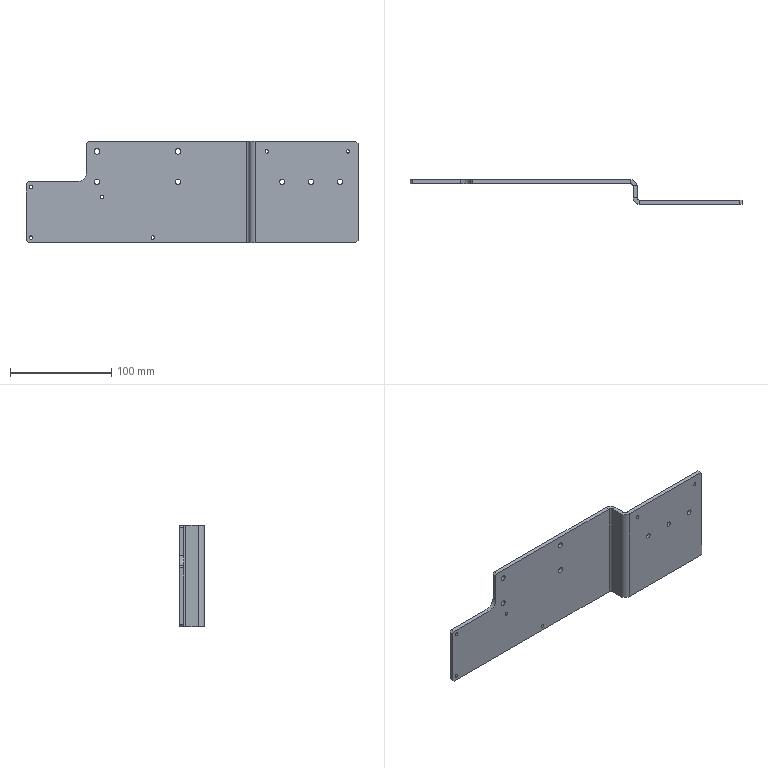Part | NX | features BREP 1 | 1 solid | 56 faces | box 327.5 x 24 x 100 mm | volume 127251 mm3 | cylinder 31 | plane 25 | commonest cylinder face diameters 3.3 x12 5.5 x8 5 x6 4 x2 12 x2 20 x1